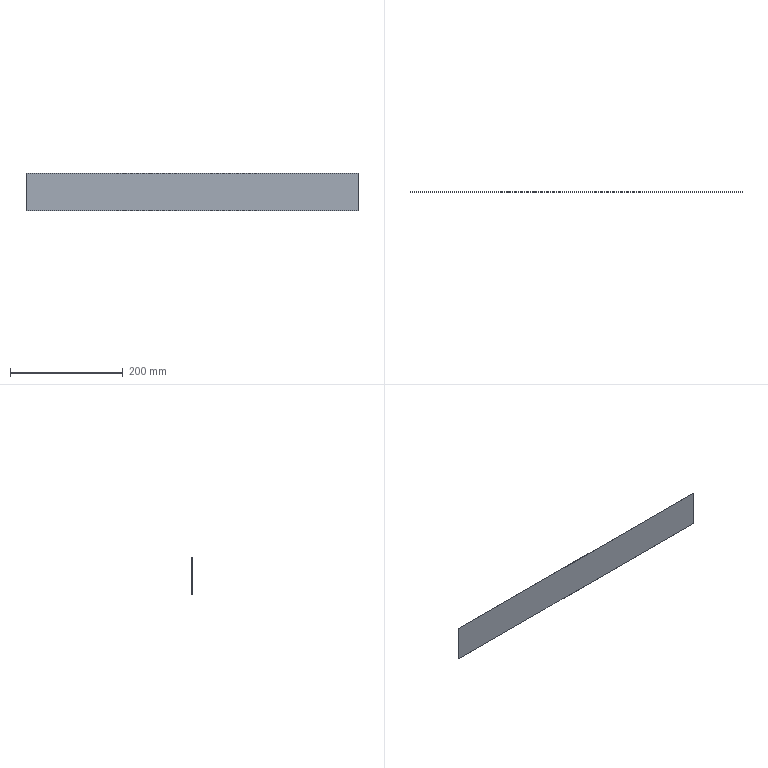Part | SolidWorks | features BaseBody 1 | 1 solid | 6 faces | box 590 x 0.2 x 66 mm | volume 7788 mm3 | plane 6
STEP:
#1=CARTESIAN_POINT('',(301.479,1879.744,-105.5));
#2=VERTEX_POINT('',#1);
#3=CARTESIAN_POINT('',(-288.521,1879.744,-105.5));
#4=VERTEX_POINT('',#3);
#5=CARTESIAN_POINT('',(-288.521,1879.744,-105.5));
#6=DIRECTION('',(-1.,0.,0.));
#7=VECTOR('',#6,1000.);
#8=LINE('',#5,#7);
#9=EDGE_CURVE('',#2,#4,#8,.T.);
#10=ORIENTED_EDGE('',*,*,#9,.T.);
#11=CARTESIAN_POINT('',(-288.521,1879.744,-39.5));
#12=VERTEX_POINT('',#11);
#13=CARTESIAN_POINT('',(-288.521,1879.744,-39.5));
#14=DIRECTION('',(0.,0.,1.));
#15=VECTOR('',#14,1000.);
#16=LINE('',#13,#15);
#17=EDGE_CURVE('',#4,#12,#16,.T.);
#18=ORIENTED_EDGE('',*,*,#17,.T.);
#19=CARTESIAN_POINT('',(301.479,1879.744,-39.5));
#20=VERTEX_POINT('',#19);
#21=CARTESIAN_POINT('',(-288.521,1879.744,-39.5));
#22=DIRECTION('',(1.,0.,0.));
#23=VECTOR('',#22,1000.);
#24=LINE('',#21,#23);
#25=EDGE_CURVE('',#12,#20,#24,.T.);
#26=ORIENTED_EDGE('',*,*,#25,.T.);
#27=CARTESIAN_POINT('',(301.479,1879.744,-39.5));
#28=DIRECTION('',(0.,0.,-1.));
#29=VECTOR('',#28,1000.);
#30=LINE('',#27,#29);
#31=EDGE_CURVE('',#20,#2,#30,.T.);
#32=ORIENTED_EDGE('',*,*,#31,.T.);
#33=EDGE_LOOP('',(#10,#18,#26,#32));
#34=FACE_OUTER_BOUND('',#33,.T.);
#35=CARTESIAN_POINT('',(-288.521,1879.744,-39.5));
#36=DIRECTION('',(0.,1.,0.));
#37=DIRECTION('',(0.,0.,1.));
#38=AXIS2_PLACEMENT_3D('',#35,#36,#37);
#39=PLANE('',#38);
#40=ADVANCED_FACE('',(#34),#39,.T.);
#41=CARTESIAN_POINT('',(-288.521,1879.544,-39.5));
#42=VERTEX_POINT('',#41);
#43=CARTESIAN_POINT('',(-288.521,1879.644,-39.5));
#44=DIRECTION('',(0.,-1.,0.));
#45=VECTOR('',#44,1000.);
#46=LINE('',#43,#45);
#47=EDGE_CURVE('',#12,#42,#46,.T.);
#48=ORIENTED_EDGE('',*,*,#47,.F.);
#49=ORIENTED_EDGE('',*,*,#17,.F.);
#50=CARTESIAN_POINT('',(-288.521,1879.544,-105.5));
#51=VERTEX_POINT('',#50);
#52=CARTESIAN_POINT('',(-288.521,1879.644,-105.5));
#53=DIRECTION('',(0.,1.,0.));
#54=VECTOR('',#53,1000.);
#55=LINE('',#52,#54);
#56=EDGE_CURVE('',#51,#4,#55,.T.);
#57=ORIENTED_EDGE('',*,*,#56,.F.);
#58=CARTESIAN_POINT('',(-288.521,1879.544,-72.5));
#59=DIRECTION('',(0.,0.,-1.));
#60=VECTOR('',#59,1000.);
#61=LINE('',#58,#60);
#62=EDGE_CURVE('',#42,#51,#61,.T.);
#63=ORIENTED_EDGE('',*,*,#62,.F.);
#64=EDGE_LOOP('',(#48,#49,#57,#63));
#65=FACE_OUTER_BOUND('',#64,.T.);
#66=CARTESIAN_POINT('',(-288.521,1879.644,-72.5));
#67=DIRECTION('',(1.,0.,0.));
#68=DIRECTION('',(0.,0.,-1.));
#69=AXIS2_PLACEMENT_3D('',#66,#67,#68);
#70=PLANE('',#69);
#71=ADVANCED_FACE('',(#65),#70,.F.);
#72=CARTESIAN_POINT('',(301.479,1879.544,-105.5));
#73=VERTEX_POINT('',#72);
#74=CARTESIAN_POINT('',(-288.521,1879.544,-105.5));
#75=DIRECTION('',(-1.,0.,0.));
#76=VECTOR('',#75,1000.);
#77=LINE('',#74,#76);
#78=EDGE_CURVE('',#73,#51,#77,.T.);
#79=ORIENTED_EDGE('',*,*,#78,.T.);
#80=ORIENTED_EDGE('',*,*,#56,.T.);
#81=ORIENTED_EDGE('',*,*,#9,.F.);
#82=CARTESIAN_POINT('',(301.479,1879.744,-105.5));
#83=DIRECTION('',(0.,-1.,0.));
#84=VECTOR('',#83,1000.);
#85=LINE('',#82,#84);
#86=EDGE_CURVE('',#2,#73,#85,.T.);
#87=ORIENTED_EDGE('',*,*,#86,.T.);
#88=EDGE_LOOP('',(#79,#80,#81,#87));
#89=FACE_OUTER_BOUND('',#88,.T.);
#90=CARTESIAN_POINT('',(-288.521,1879.744,-105.5));
#91=DIRECTION('',(0.,0.,-1.));
#92=DIRECTION('',(-1.,0.,0.));
#93=AXIS2_PLACEMENT_3D('',#90,#91,#92);
#94=PLANE('',#93);
#95=ADVANCED_FACE('',(#89),#94,.T.);
#96=ORIENTED_EDGE('',*,*,#31,.F.);
#97=CARTESIAN_POINT('',(301.479,1879.544,-39.5));
#98=VERTEX_POINT('',#97);
#99=CARTESIAN_POINT('',(301.479,1879.644,-39.5));
#100=DIRECTION('',(0.,-1.,0.));
#101=VECTOR('',#100,1000.);
#102=LINE('',#99,#101);
#103=EDGE_CURVE('',#20,#98,#102,.T.);
#104=ORIENTED_EDGE('',*,*,#103,.T.);
#105=CARTESIAN_POINT('',(301.479,1879.544,-72.5));
#106=DIRECTION('',(0.,0.,-1.));
#107=VECTOR('',#106,1000.);
#108=LINE('',#105,#107);
#109=EDGE_CURVE('',#98,#73,#108,.T.);
#110=ORIENTED_EDGE('',*,*,#109,.T.);
#111=ORIENTED_EDGE('',*,*,#86,.F.);
#112=EDGE_LOOP('',(#96,#104,#110,#111));
#113=FACE_OUTER_BOUND('',#112,.T.);
#114=CARTESIAN_POINT('',(301.479,1879.644,-72.5));
#115=DIRECTION('',(1.,0.,0.));
#116=DIRECTION('',(0.,0.,-1.));
#117=AXIS2_PLACEMENT_3D('',#114,#115,#116);
#118=PLANE('',#117);
#119=ADVANCED_FACE('',(#113),#118,.T.);
#120=ORIENTED_EDGE('',*,*,#25,.F.);
#121=ORIENTED_EDGE('',*,*,#47,.T.);
#122=CARTESIAN_POINT('',(-288.521,1879.544,-39.5));
#123=DIRECTION('',(1.,0.,0.));
#124=VECTOR('',#123,1000.);
#125=LINE('',#122,#124);
#126=EDGE_CURVE('',#42,#98,#125,.T.);
#127=ORIENTED_EDGE('',*,*,#126,.T.);
#128=ORIENTED_EDGE('',*,*,#103,.F.);
#129=EDGE_LOOP('',(#120,#121,#127,#128));
#130=FACE_OUTER_BOUND('',#129,.T.);
#131=CARTESIAN_POINT('',(-288.521,1879.544,-39.5));
#132=DIRECTION('',(0.,0.,1.));
#133=DIRECTION('',(1.,0.,0.));
#134=AXIS2_PLACEMENT_3D('',#131,#132,#133);
#135=PLANE('',#134);
#136=ADVANCED_FACE('',(#130),#135,.T.);
#137=ORIENTED_EDGE('',*,*,#126,.F.);
#138=ORIENTED_EDGE('',*,*,#62,.T.);
#139=ORIENTED_EDGE('',*,*,#78,.F.);
#140=ORIENTED_EDGE('',*,*,#109,.F.);
#141=EDGE_LOOP('',(#137,#138,#139,#140));
#142=FACE_OUTER_BOUND('',#141,.T.);
#143=CARTESIAN_POINT('',(-288.521,1879.544,-105.5));
#144=DIRECTION('',(0.,-1.,0.));
#145=DIRECTION('',(0.,0.,-1.));
#146=AXIS2_PLACEMENT_3D('',#143,#144,#145);
#147=PLANE('',#146);
#148=ADVANCED_FACE('',(#142),#147,.T.);
#149=CLOSED_SHELL('',(#40,#71,#95,#119,#136,#148));
#150=MANIFOLD_SOLID_BREP('',#149);
#151=CARTESIAN_POINT('',(0.,0.,0.));
#152=DIRECTION('',(0.,0.,1.));
#153=DIRECTION('',(1.,0.,0.));
#154=AXIS2_PLACEMENT_3D('',#151,#152,#153);
#155=(LENGTH_UNIT()NAMED_UNIT(*)SI_UNIT(.MILLI.,.METRE.));
#156=UNCERTAINTY_MEASURE_WITH_UNIT(LENGTH_MEASURE(0.00001),#155,'','');
#157=(NAMED_UNIT(*)PLANE_ANGLE_UNIT()SI_UNIT($,.RADIAN.));
#158=(NAMED_UNIT(*)SI_UNIT($,.STERADIAN.)SOLID_ANGLE_UNIT());
#159=(GEOMETRIC_REPRESENTATION_CONTEXT(3)GLOBAL_UNCERTAINTY_ASSIGNED_CONTEXT((#156))GLOBAL_UNIT_ASSIGNED_CONTEXT((#155,#157,#158))REPRESENTATION_CONTEXT('',''));
#160=ADVANCED_BREP_SHAPE_REPRESENTATION('',(#150,#154),#159);